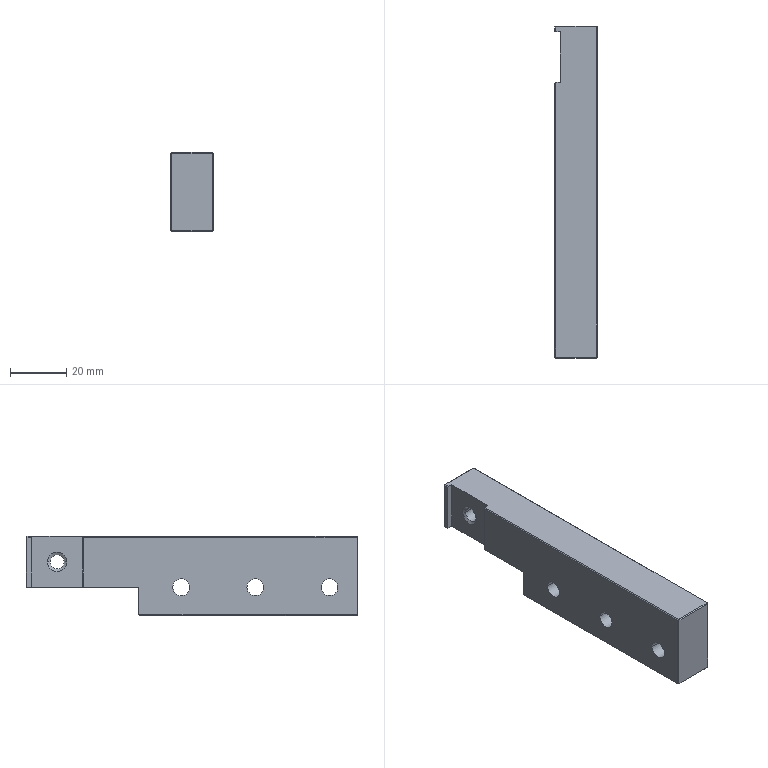Part | NX | 1 solid | 37 faces | box 15 x 117.567 x 28 mm | volume 41173 mm3 | plane 27 | cylinder 8 | cone 2 | commonest cylinder face diameters 6 x6 5 x2
STEP:
#1=CARTESIAN_POINT('',(-190.3,-54.817,-9.2));
#2=VERTEX_POINT('',#1);
#3=CARTESIAN_POINT('',(-204.7,-54.817,-9.2));
#4=VERTEX_POINT('',#3);
#5=CARTESIAN_POINT('',(-197.5,-54.817,-9.2));
#6=DIRECTION('',(-1.,0.,0.));
#7=VECTOR('',#6,1000.);
#8=LINE('',#5,#7);
#9=EDGE_CURVE('',#2,#4,#8,.T.);
#10=ORIENTED_EDGE('',*,*,#9,.F.);
#11=CARTESIAN_POINT('',(-190.3,-54.817,18.2));
#12=VERTEX_POINT('',#11);
#13=CARTESIAN_POINT('',(-190.3,-54.817,4.5));
#14=DIRECTION('',(0.,0.,-1.));
#15=VECTOR('',#14,1000.);
#16=LINE('',#13,#15);
#17=EDGE_CURVE('',#12,#2,#16,.T.);
#18=ORIENTED_EDGE('',*,*,#17,.F.);
#19=CARTESIAN_POINT('',(-204.7,-54.817,18.2));
#20=VERTEX_POINT('',#19);
#21=CARTESIAN_POINT('',(-197.5,-54.817,18.2));
#22=DIRECTION('',(-1.,0.,0.));
#23=VECTOR('',#22,1000.);
#24=LINE('',#21,#23);
#25=EDGE_CURVE('',#12,#20,#24,.T.);
#26=ORIENTED_EDGE('',*,*,#25,.T.);
#27=CARTESIAN_POINT('',(-204.7,-54.817,4.5));
#28=DIRECTION('',(0.,0.,-1.));
#29=VECTOR('',#28,1000.);
#30=LINE('',#27,#29);
#31=EDGE_CURVE('',#20,#4,#30,.T.);
#32=ORIENTED_EDGE('',*,*,#31,.T.);
#33=EDGE_LOOP('',(#10,#18,#26,#32));
#34=FACE_BOUND('',#33,.T.);
#35=CARTESIAN_POINT('',(-190.,-54.817,10.5));
#36=DIRECTION('',(0.,-1.,0.));
#37=DIRECTION('',(0.,0.,-1.));
#38=AXIS2_PLACEMENT_3D('',#35,#36,#37);
#39=PLANE('',#38);
#40=ADVANCED_FACE('',(#34),#39,.T.);
#41=CARTESIAN_POINT('',(-190.3,-54.517,18.5));
#42=VERTEX_POINT('',#41);
#43=CARTESIAN_POINT('',(-190.3,62.45,18.5));
#44=VERTEX_POINT('',#43);
#45=CARTESIAN_POINT('',(-190.3,3.967,18.5));
#46=DIRECTION('',(0.,1.,0.));
#47=VECTOR('',#46,1000.);
#48=LINE('',#45,#47);
#49=EDGE_CURVE('',#42,#44,#48,.T.);
#50=ORIENTED_EDGE('',*,*,#49,.T.);
#51=CARTESIAN_POINT('',(-204.7,62.45,18.5));
#52=VERTEX_POINT('',#51);
#53=CARTESIAN_POINT('',(-197.5,62.45,18.5));
#54=DIRECTION('',(1.,0.,0.));
#55=VECTOR('',#54,1000.);
#56=LINE('',#53,#55);
#57=EDGE_CURVE('',#52,#44,#56,.T.);
#58=ORIENTED_EDGE('',*,*,#57,.F.);
#59=CARTESIAN_POINT('',(-204.7,60.75,18.5));
#60=VERTEX_POINT('',#59);
#61=CARTESIAN_POINT('',(-204.7,61.75,18.5));
#62=DIRECTION('',(0.,1.,0.));
#63=VECTOR('',#62,1000.);
#64=LINE('',#61,#63);
#65=EDGE_CURVE('',#60,#52,#64,.T.);
#66=ORIENTED_EDGE('',*,*,#65,.F.);
#67=CARTESIAN_POINT('',(-203.,60.75,18.5));
#68=VERTEX_POINT('',#67);
#69=CARTESIAN_POINT('',(-190.,60.75,18.5));
#70=DIRECTION('',(-1.,0.,0.));
#71=VECTOR('',#70,1000.);
#72=LINE('',#69,#71);
#73=EDGE_CURVE('',#68,#60,#72,.T.);
#74=ORIENTED_EDGE('',*,*,#73,.F.);
#75=CARTESIAN_POINT('',(-203.,42.75,18.5));
#76=VERTEX_POINT('',#75);
#77=CARTESIAN_POINT('',(-203.,21.496,18.5));
#78=DIRECTION('',(0.,-1.,0.));
#79=VECTOR('',#78,1000.);
#80=LINE('',#77,#79);
#81=EDGE_CURVE('',#68,#76,#80,.T.);
#82=ORIENTED_EDGE('',*,*,#81,.T.);
#83=CARTESIAN_POINT('',(-204.7,42.75,18.5));
#84=VERTEX_POINT('',#83);
#85=CARTESIAN_POINT('',(-190.,42.75,18.5));
#86=DIRECTION('',(1.,0.,0.));
#87=VECTOR('',#86,1000.);
#88=LINE('',#85,#87);
#89=EDGE_CURVE('',#84,#76,#88,.T.);
#90=ORIENTED_EDGE('',*,*,#89,.F.);
#91=CARTESIAN_POINT('',(-204.7,-54.517,18.5));
#92=VERTEX_POINT('',#91);
#93=CARTESIAN_POINT('',(-204.7,-6.033,18.5));
#94=DIRECTION('',(0.,1.,0.));
#95=VECTOR('',#94,1000.);
#96=LINE('',#93,#95);
#97=EDGE_CURVE('',#92,#84,#96,.T.);
#98=ORIENTED_EDGE('',*,*,#97,.F.);
#99=CARTESIAN_POINT('',(-197.5,-54.517,18.5));
#100=DIRECTION('',(-1.,0.,0.));
#101=VECTOR('',#100,1000.);
#102=LINE('',#99,#101);
#103=EDGE_CURVE('',#42,#92,#102,.T.);
#104=ORIENTED_EDGE('',*,*,#103,.F.);
#105=EDGE_LOOP('',(#50,#58,#66,#74,#82,#90,#98,#104));
#106=FACE_BOUND('',#105,.T.);
#107=CARTESIAN_POINT('',(-190.,42.75,18.5));
#108=DIRECTION('',(0.,0.,1.));
#109=DIRECTION('',(1.,0.,0.));
#110=AXIS2_PLACEMENT_3D('',#107,#108,#109);
#111=PLANE('',#110);
#112=ADVANCED_FACE('',(#106),#111,.T.);
#113=CARTESIAN_POINT('',(-205.,22.75,-9.2));
#114=VERTEX_POINT('',#113);
#115=CARTESIAN_POINT('',(-190.,22.75,-9.2));
#116=VERTEX_POINT('',#115);
#117=CARTESIAN_POINT('',(-197.5,22.75,-9.2));
#118=DIRECTION('',(1.,0.,0.));
#119=VECTOR('',#118,1000.);
#120=LINE('',#117,#119);
#121=EDGE_CURVE('',#114,#116,#120,.T.);
#122=ORIENTED_EDGE('',*,*,#121,.F.);
#123=CARTESIAN_POINT('',(-205.,22.75,0.5));
#124=VERTEX_POINT('',#123);
#125=CARTESIAN_POINT('',(-205.,22.75,29.147));
#126=DIRECTION('',(0.,0.,-1.));
#127=VECTOR('',#126,1000.);
#128=LINE('',#125,#127);
#129=EDGE_CURVE('',#124,#114,#128,.T.);
#130=ORIENTED_EDGE('',*,*,#129,.F.);
#131=CARTESIAN_POINT('',(-190.,22.75,0.5));
#132=VERTEX_POINT('',#131);
#133=CARTESIAN_POINT('',(-190.,22.75,0.5));
#134=DIRECTION('',(1.,0.,0.));
#135=VECTOR('',#134,1000.);
#136=LINE('',#133,#135);
#137=EDGE_CURVE('',#124,#132,#136,.T.);
#138=ORIENTED_EDGE('',*,*,#137,.T.);
#139=CARTESIAN_POINT('',(-190.,22.75,29.147));
#140=DIRECTION('',(0.,0.,-1.));
#141=VECTOR('',#140,1000.);
#142=LINE('',#139,#141);
#143=EDGE_CURVE('',#132,#116,#142,.T.);
#144=ORIENTED_EDGE('',*,*,#143,.T.);
#145=EDGE_LOOP('',(#122,#130,#138,#144));
#146=FACE_BOUND('',#145,.T.);
#147=CARTESIAN_POINT('',(-190.,22.75,-9.5));
#148=DIRECTION('',(0.,1.,0.));
#149=DIRECTION('',(1.,0.,0.));
#150=AXIS2_PLACEMENT_3D('',#147,#148,#149);
#151=PLANE('',#150);
#152=ADVANCED_FACE('',(#146),#151,.T.);
#153=CARTESIAN_POINT('',(-190.3,-54.517,-9.5));
#154=VERTEX_POINT('',#153);
#155=CARTESIAN_POINT('',(-190.3,22.45,-9.5));
#156=VERTEX_POINT('',#155);
#157=CARTESIAN_POINT('',(-190.3,-16.033,-9.5));
#158=DIRECTION('',(0.,1.,0.));
#159=VECTOR('',#158,1000.);
#160=LINE('',#157,#159);
#161=EDGE_CURVE('',#154,#156,#160,.T.);
#162=ORIENTED_EDGE('',*,*,#161,.F.);
#163=CARTESIAN_POINT('',(-204.7,-54.517,-9.5));
#164=VERTEX_POINT('',#163);
#165=CARTESIAN_POINT('',(-197.5,-54.517,-9.5));
#166=DIRECTION('',(-1.,0.,0.));
#167=VECTOR('',#166,1000.);
#168=LINE('',#165,#167);
#169=EDGE_CURVE('',#154,#164,#168,.T.);
#170=ORIENTED_EDGE('',*,*,#169,.T.);
#171=CARTESIAN_POINT('',(-204.7,22.45,-9.5));
#172=VERTEX_POINT('',#171);
#173=CARTESIAN_POINT('',(-204.7,-16.033,-9.5));
#174=DIRECTION('',(0.,1.,0.));
#175=VECTOR('',#174,1000.);
#176=LINE('',#173,#175);
#177=EDGE_CURVE('',#164,#172,#176,.T.);
#178=ORIENTED_EDGE('',*,*,#177,.T.);
#179=CARTESIAN_POINT('',(-197.5,22.45,-9.5));
#180=DIRECTION('',(1.,0.,0.));
#181=VECTOR('',#180,1000.);
#182=LINE('',#179,#181);
#183=EDGE_CURVE('',#172,#156,#182,.T.);
#184=ORIENTED_EDGE('',*,*,#183,.T.);
#185=EDGE_LOOP('',(#162,#170,#178,#184));
#186=FACE_BOUND('',#185,.T.);
#187=CARTESIAN_POINT('',(-190.,-54.817,-9.5));
#188=DIRECTION('',(0.,0.,-1.));
#189=DIRECTION('',(0.,-1.,0.));
#190=AXIS2_PLACEMENT_3D('',#187,#188,#189);
#191=PLANE('',#190);
#192=ADVANCED_FACE('',(#186),#191,.T.);
#193=ORIENTED_EDGE('',*,*,#137,.F.);
#194=CARTESIAN_POINT('',(-205.,42.45,0.5));
#195=VERTEX_POINT('',#194);
#196=CARTESIAN_POINT('',(-205.,21.496,0.5));
#197=DIRECTION('',(0.,1.,0.));
#198=VECTOR('',#197,1000.);
#199=LINE('',#196,#198);
#200=EDGE_CURVE('',#124,#195,#199,.T.);
#201=ORIENTED_EDGE('',*,*,#200,.T.);
#202=CARTESIAN_POINT('',(-204.7,42.75,0.5));
#203=VERTEX_POINT('',#202);
#204=CARTESIAN_POINT('',(-190.,57.45,0.5));
#205=DIRECTION('',(0.7071,0.7071,0.));
#206=VECTOR('',#205,1000.);
#207=LINE('',#204,#206);
#208=EDGE_CURVE('',#195,#203,#207,.T.);
#209=ORIENTED_EDGE('',*,*,#208,.T.);
#210=CARTESIAN_POINT('',(-203.,42.75,0.5));
#211=VERTEX_POINT('',#210);
#212=CARTESIAN_POINT('',(-190.,42.75,0.5));
#213=DIRECTION('',(-1.,0.,0.));
#214=VECTOR('',#213,1000.);
#215=LINE('',#212,#214);
#216=EDGE_CURVE('',#211,#203,#215,.T.);
#217=ORIENTED_EDGE('',*,*,#216,.F.);
#218=CARTESIAN_POINT('',(-203.,60.75,0.5));
#219=VERTEX_POINT('',#218);
#220=CARTESIAN_POINT('',(-203.,21.496,0.5));
#221=DIRECTION('',(0.,1.,0.));
#222=VECTOR('',#221,1000.);
#223=LINE('',#220,#222);
#224=EDGE_CURVE('',#211,#219,#223,.T.);
#225=ORIENTED_EDGE('',*,*,#224,.T.);
#226=CARTESIAN_POINT('',(-205.,60.75,0.5));
#227=VERTEX_POINT('',#226);
#228=CARTESIAN_POINT('',(-190.,60.75,0.5));
#229=DIRECTION('',(1.,0.,0.));
#230=VECTOR('',#229,1000.);
#231=LINE('',#228,#230);
#232=EDGE_CURVE('',#227,#219,#231,.T.);
#233=ORIENTED_EDGE('',*,*,#232,.F.);
#234=CARTESIAN_POINT('',(-205.,62.45,0.5));
#235=VERTEX_POINT('',#234);
#236=CARTESIAN_POINT('',(-205.,21.496,0.5));
#237=DIRECTION('',(0.,1.,0.));
#238=VECTOR('',#237,1000.);
#239=LINE('',#236,#238);
#240=EDGE_CURVE('',#227,#235,#239,.T.);
#241=ORIENTED_EDGE('',*,*,#240,.T.);
#242=CARTESIAN_POINT('',(-190.,62.45,0.5));
#243=VERTEX_POINT('',#242);
#244=CARTESIAN_POINT('',(-197.5,62.45,0.5));
#245=DIRECTION('',(1.,0.,0.));
#246=VECTOR('',#245,1000.);
#247=LINE('',#244,#246);
#248=EDGE_CURVE('',#235,#243,#247,.T.);
#249=ORIENTED_EDGE('',*,*,#248,.T.);
#250=CARTESIAN_POINT('',(-190.,21.496,0.5));
#251=DIRECTION('',(0.,1.,0.));
#252=VECTOR('',#251,1000.);
#253=LINE('',#250,#252);
#254=EDGE_CURVE('',#132,#243,#253,.T.);
#255=ORIENTED_EDGE('',*,*,#254,.F.);
#256=EDGE_LOOP('',(#193,#201,#209,#217,#225,#233,#241,#249,#255));
#257=FACE_BOUND('',#256,.T.);
#258=CARTESIAN_POINT('',(-205.,42.75,0.5));
#259=DIRECTION('',(0.,0.,-1.));
#260=DIRECTION('',(0.,-1.,0.));
#261=AXIS2_PLACEMENT_3D('',#258,#259,#260);
#262=PLANE('',#261);
#263=ADVANCED_FACE('',(#257),#262,.T.);
#264=CARTESIAN_POINT('',(-190.3,62.75,18.2));
#265=VERTEX_POINT('',#264);
#266=CARTESIAN_POINT('',(-190.3,62.75,0.8));
#267=VERTEX_POINT('',#266);
#268=CARTESIAN_POINT('',(-190.3,62.75,9.5));
#269=DIRECTION('',(0.,0.,-1.));
#270=VECTOR('',#269,1000.);
#271=LINE('',#268,#270);
#272=EDGE_CURVE('',#265,#267,#271,.T.);
#273=ORIENTED_EDGE('',*,*,#272,.T.);
#274=CARTESIAN_POINT('',(-204.7,62.75,0.8));
#275=VERTEX_POINT('',#274);
#276=CARTESIAN_POINT('',(-197.5,62.75,0.8));
#277=DIRECTION('',(1.,0.,0.));
#278=VECTOR('',#277,1000.);
#279=LINE('',#276,#278);
#280=EDGE_CURVE('',#275,#267,#279,.T.);
#281=ORIENTED_EDGE('',*,*,#280,.F.);
#282=CARTESIAN_POINT('',(-204.7,62.75,18.2));
#283=VERTEX_POINT('',#282);
#284=CARTESIAN_POINT('',(-204.7,62.75,9.5));
#285=DIRECTION('',(0.,0.,-1.));
#286=VECTOR('',#285,1000.);
#287=LINE('',#284,#286);
#288=EDGE_CURVE('',#283,#275,#287,.T.);
#289=ORIENTED_EDGE('',*,*,#288,.F.);
#290=CARTESIAN_POINT('',(-197.5,62.75,18.2));
#291=DIRECTION('',(1.,0.,0.));
#292=VECTOR('',#291,1000.);
#293=LINE('',#290,#292);
#294=EDGE_CURVE('',#283,#265,#293,.T.);
#295=ORIENTED_EDGE('',*,*,#294,.T.);
#296=EDGE_LOOP('',(#273,#281,#289,#295));
#297=FACE_BOUND('',#296,.T.);
#298=CARTESIAN_POINT('',(-198.847,62.75,5.404));
#299=DIRECTION('',(0.,1.,0.));
#300=DIRECTION('',(1.,0.,0.));
#301=AXIS2_PLACEMENT_3D('',#298,#299,#300);
#302=PLANE('',#301);
#303=ADVANCED_FACE('',(#297),#302,.T.);
#304=ORIENTED_EDGE('',*,*,#232,.T.);
#305=CARTESIAN_POINT('',(-203.,60.75,18.5));
#306=DIRECTION('',(0.,0.,-1.));
#307=VECTOR('',#306,1000.);
#308=LINE('',#305,#307);
#309=EDGE_CURVE('',#68,#219,#308,.T.);
#310=ORIENTED_EDGE('',*,*,#309,.F.);
#311=ORIENTED_EDGE('',*,*,#73,.T.);
#312=CARTESIAN_POINT('',(-205.,60.75,18.2));
#313=VERTEX_POINT('',#312);
#314=CARTESIAN_POINT('',(-190.,60.75,33.2));
#315=DIRECTION('',(-0.7071,0.,-0.7071));
#316=VECTOR('',#315,1000.);
#317=LINE('',#314,#316);
#318=EDGE_CURVE('',#60,#313,#317,.T.);
#319=ORIENTED_EDGE('',*,*,#318,.T.);
#320=CARTESIAN_POINT('',(-205.,60.75,29.147));
#321=DIRECTION('',(0.,0.,-1.));
#322=VECTOR('',#321,1000.);
#323=LINE('',#320,#322);
#324=EDGE_CURVE('',#313,#227,#323,.T.);
#325=ORIENTED_EDGE('',*,*,#324,.T.);
#326=EDGE_LOOP('',(#304,#310,#311,#319,#325));
#327=FACE_BOUND('',#326,.T.);
#328=CARTESIAN_POINT('',(-205.,60.75,18.5));
#329=DIRECTION('',(0.,1.,0.));
#330=DIRECTION('',(1.,0.,0.));
#331=AXIS2_PLACEMENT_3D('',#328,#329,#330);
#332=PLANE('',#331);
#333=ADVANCED_FACE('',(#327),#332,.F.);
#334=ORIENTED_EDGE('',*,*,#309,.T.);
#335=ORIENTED_EDGE('',*,*,#224,.F.);
#336=CARTESIAN_POINT('',(-203.,42.75,0.5));
#337=DIRECTION('',(0.,0.,1.));
#338=VECTOR('',#337,1000.);
#339=LINE('',#336,#338);
#340=EDGE_CURVE('',#211,#76,#339,.T.);
#341=ORIENTED_EDGE('',*,*,#340,.T.);
#342=ORIENTED_EDGE('',*,*,#81,.F.);
#343=EDGE_LOOP('',(#334,#335,#341,#342));
#344=FACE_BOUND('',#343,.T.);
#345=CARTESIAN_POINT('',(-203.,55.2,9.5));
#346=VERTEX_POINT('',#345);
#347=CARTESIAN_POINT('',(-203.,48.3,9.5));
#348=VERTEX_POINT('',#347);
#349=CARTESIAN_POINT('',(-203.,51.75,9.5));
#350=DIRECTION('',(-1.,0.,0.));
#351=DIRECTION('',(0.,-1.,0.));
#352=AXIS2_PLACEMENT_3D('',#349,#350,#351);
#353=CIRCLE('',#352,3.45);
#354=EDGE_CURVE('',#346,#348,#353,.T.);
#355=ORIENTED_EDGE('',*,*,#354,.F.);
#356=CARTESIAN_POINT('',(-203.,51.75,9.5));
#357=DIRECTION('',(-1.,0.,0.));
#358=DIRECTION('',(0.,-1.,0.));
#359=AXIS2_PLACEMENT_3D('',#356,#357,#358);
#360=CIRCLE('',#359,3.45);
#361=EDGE_CURVE('',#348,#346,#360,.T.);
#362=ORIENTED_EDGE('',*,*,#361,.F.);
#363=EDGE_LOOP('',(#355,#362));
#364=FACE_BOUND('',#363,.T.);
#365=CARTESIAN_POINT('',(-203.,52.251,12.817));
#366=DIRECTION('',(-1.,0.,0.));
#367=DIRECTION('',(0.,0.,1.));
#368=AXIS2_PLACEMENT_3D('',#365,#366,#367);
#369=PLANE('',#368);
#370=ADVANCED_FACE('',(#344,#364),#369,.T.);
#371=ORIENTED_EDGE('',*,*,#89,.T.);
#372=ORIENTED_EDGE('',*,*,#340,.F.);
#373=ORIENTED_EDGE('',*,*,#216,.T.);
#374=CARTESIAN_POINT('',(-204.7,42.75,9.5));
#375=DIRECTION('',(0.,0.,1.));
#376=VECTOR('',#375,1000.);
#377=LINE('',#374,#376);
#378=EDGE_CURVE('',#203,#84,#377,.T.);
#379=ORIENTED_EDGE('',*,*,#378,.T.);
#380=EDGE_LOOP('',(#371,#372,#373,#379));
#381=FACE_BOUND('',#380,.T.);
#382=CARTESIAN_POINT('',(-205.,42.75,0.5));
#383=DIRECTION('',(0.,-1.,0.));
#384=DIRECTION('',(0.,0.,-1.));
#385=AXIS2_PLACEMENT_3D('',#382,#383,#384);
#386=PLANE('',#385);
#387=ADVANCED_FACE('',(#381),#386,.F.);
#388=CARTESIAN_POINT('',(-202.452,54.25,9.5));
#389=VERTEX_POINT('',#388);
#390=CARTESIAN_POINT('',(-202.452,49.25,9.5));
#391=VERTEX_POINT('',#390);
#392=CARTESIAN_POINT('',(-202.452,51.75,9.5));
#393=DIRECTION('',(-1.,0.,0.));
#394=DIRECTION('',(0.,-1.,0.));
#395=AXIS2_PLACEMENT_3D('',#392,#393,#394);
#396=CIRCLE('',#395,2.5);
#397=EDGE_CURVE('',#389,#391,#396,.T.);
#398=ORIENTED_EDGE('',*,*,#397,.T.);
#399=CARTESIAN_POINT('',(-190.,49.25,9.5));
#400=VERTEX_POINT('',#399);
#401=CARTESIAN_POINT('',(-203.,49.25,9.5));
#402=DIRECTION('',(-1.,0.,0.));
#403=VECTOR('',#402,1000.);
#404=LINE('',#401,#403);
#405=EDGE_CURVE('',#391,#400,#404,.F.);
#406=ORIENTED_EDGE('',*,*,#405,.T.);
#407=CARTESIAN_POINT('',(-190.,54.25,9.5));
#408=VERTEX_POINT('',#407);
#409=CARTESIAN_POINT('',(-190.,51.75,9.5));
#410=DIRECTION('',(-1.,0.,0.));
#411=DIRECTION('',(0.,-1.,0.));
#412=AXIS2_PLACEMENT_3D('',#409,#410,#411);
#413=CIRCLE('',#412,2.5);
#414=EDGE_CURVE('',#408,#400,#413,.T.);
#415=ORIENTED_EDGE('',*,*,#414,.F.);
#416=CARTESIAN_POINT('',(-203.,54.25,9.5));
#417=DIRECTION('',(-1.,0.,0.));
#418=VECTOR('',#417,1000.);
#419=LINE('',#416,#418);
#420=EDGE_CURVE('',#389,#408,#419,.F.);
#421=ORIENTED_EDGE('',*,*,#420,.F.);
#422=EDGE_LOOP('',(#398,#406,#415,#421));
#423=FACE_BOUND('',#422,.T.);
#424=CARTESIAN_POINT('',(-203.,51.75,9.5));
#425=DIRECTION('',(-1.,0.,0.));
#426=DIRECTION('',(0.,-1.,0.));
#427=AXIS2_PLACEMENT_3D('',#424,#425,#426);
#428=CYLINDRICAL_SURFACE('',#427,2.5);
#429=ADVANCED_FACE('',(#423),#428,.F.);
#430=ORIENTED_EDGE('',*,*,#397,.F.);
#431=CARTESIAN_POINT('',(-202.452,54.25,9.5));
#432=DIRECTION('',(-0.5,0.866,0.));
#433=VECTOR('',#432,1000.);
#434=LINE('',#431,#433);
#435=EDGE_CURVE('',#346,#389,#434,.F.);
#436=ORIENTED_EDGE('',*,*,#435,.F.);
#437=ORIENTED_EDGE('',*,*,#354,.T.);
#438=CARTESIAN_POINT('',(-202.452,49.25,9.5));
#439=DIRECTION('',(-0.5,-0.866,0.));
#440=VECTOR('',#439,1000.);
#441=LINE('',#438,#440);
#442=EDGE_CURVE('',#348,#391,#441,.F.);
#443=ORIENTED_EDGE('',*,*,#442,.T.);
#444=EDGE_LOOP('',(#430,#436,#437,#443));
#445=FACE_BOUND('',#444,.T.);
#446=CARTESIAN_POINT('',(-202.452,51.75,9.5));
#447=DIRECTION('',(-1.,0.,0.));
#448=DIRECTION('',(0.,-1.,0.));
#449=AXIS2_PLACEMENT_3D('',#446,#447,#448);
#450=CONICAL_SURFACE('',#449,2.5,1.047);
#451=ADVANCED_FACE('',(#445),#450,.F.);
#452=ORIENTED_EDGE('',*,*,#294,.F.);
#453=CARTESIAN_POINT('',(-204.85,62.6,18.35));
#454=VERTEX_POINT('',#453);
#455=CARTESIAN_POINT('',(-190.,77.45,3.5));
#456=DIRECTION('',(0.5774,0.5774,-0.5774));
#457=VECTOR('',#456,1000.);
#458=LINE('',#455,#457);
#459=EDGE_CURVE('',#454,#283,#458,.T.);
#460=ORIENTED_EDGE('',*,*,#459,.F.);
#461=CARTESIAN_POINT('',(-194.053,51.803,29.147));
#462=DIRECTION('',(-0.5774,0.5774,-0.5774));
#463=VECTOR('',#462,1000.);
#464=LINE('',#461,#463);
#465=EDGE_CURVE('',#52,#454,#464,.T.);
#466=ORIENTED_EDGE('',*,*,#465,.F.);
#467=ORIENTED_EDGE('',*,*,#57,.T.);
#468=CARTESIAN_POINT('',(-190.15,62.6,18.35));
#469=VERTEX_POINT('',#468);
#470=CARTESIAN_POINT('',(-200.947,51.803,29.147));
#471=DIRECTION('',(-0.5774,-0.5774,0.5774));
#472=VECTOR('',#471,1000.);
#473=LINE('',#470,#472);
#474=EDGE_CURVE('',#469,#44,#473,.T.);
#475=ORIENTED_EDGE('',*,*,#474,.F.);
#476=CARTESIAN_POINT('',(-190.,62.45,18.5));
#477=DIRECTION('',(-0.5774,0.5774,-0.5774));
#478=VECTOR('',#477,1000.);
#479=LINE('',#476,#478);
#480=EDGE_CURVE('',#469,#265,#479,.T.);
#481=ORIENTED_EDGE('',*,*,#480,.T.);
#482=EDGE_LOOP('',(#452,#460,#466,#467,#475,#481));
#483=FACE_BOUND('',#482,.T.);
#484=CARTESIAN_POINT('',(-197.5,62.6,18.35));
#485=DIRECTION('',(0.,0.7071,0.7071));
#486=DIRECTION('',(1.,0.,0.));
#487=AXIS2_PLACEMENT_3D('',#484,#485,#486);
#488=PLANE('',#487);
#489=ADVANCED_FACE('',(#483),#488,.T.);
#490=ORIENTED_EDGE('',*,*,#280,.T.);
#491=CARTESIAN_POINT('',(-190.,62.45,0.5));
#492=DIRECTION('',(-0.5774,0.5774,0.5774));
#493=VECTOR('',#492,1000.);
#494=LINE('',#491,#493);
#495=EDGE_CURVE('',#243,#267,#494,.T.);
#496=ORIENTED_EDGE('',*,*,#495,.F.);
#497=ORIENTED_EDGE('',*,*,#248,.F.);
#498=CARTESIAN_POINT('',(-190.,77.45,15.5));
#499=DIRECTION('',(0.5774,0.5774,0.5774));
#500=VECTOR('',#499,1000.);
#501=LINE('',#498,#500);
#502=EDGE_CURVE('',#235,#275,#501,.T.);
#503=ORIENTED_EDGE('',*,*,#502,.T.);
#504=EDGE_LOOP('',(#490,#496,#497,#503));
#505=FACE_BOUND('',#504,.T.);
#506=CARTESIAN_POINT('',(-197.5,62.6,0.65));
#507=DIRECTION('',(0.,-0.7071,0.7071));
#508=DIRECTION('',(-1.,0.,0.));
#509=AXIS2_PLACEMENT_3D('',#506,#507,#508);
#510=PLANE('',#509);
#511=ADVANCED_FACE('',(#505),#510,.F.);
#512=ORIENTED_EDGE('',*,*,#288,.T.);
#513=ORIENTED_EDGE('',*,*,#502,.F.);
#514=CARTESIAN_POINT('',(-205.,62.45,18.2));
#515=VERTEX_POINT('',#514);
#516=CARTESIAN_POINT('',(-205.,62.45,9.5));
#517=DIRECTION('',(0.,0.,-1.));
#518=VECTOR('',#517,1000.);
#519=LINE('',#516,#518);
#520=EDGE_CURVE('',#515,#235,#519,.T.);
#521=ORIENTED_EDGE('',*,*,#520,.F.);
#522=CARTESIAN_POINT('',(-190.,77.45,33.2));
#523=DIRECTION('',(0.5774,0.5774,0.5774));
#524=VECTOR('',#523,1000.);
#525=LINE('',#522,#524);
#526=EDGE_CURVE('',#515,#454,#525,.T.);
#527=ORIENTED_EDGE('',*,*,#526,.T.);
#528=ORIENTED_EDGE('',*,*,#459,.T.);
#529=EDGE_LOOP('',(#512,#513,#521,#527,#528));
#530=FACE_BOUND('',#529,.T.);
#531=CARTESIAN_POINT('',(-204.85,62.6,9.5));
#532=DIRECTION('',(0.7071,-0.7071,0.));
#533=DIRECTION('',(0.,0.,-1.));
#534=AXIS2_PLACEMENT_3D('',#531,#532,#533);
#535=PLANE('',#534);
#536=ADVANCED_FACE('',(#530),#535,.F.);
#537=ORIENTED_EDGE('',*,*,#272,.F.);
#538=ORIENTED_EDGE('',*,*,#480,.F.);
#539=CARTESIAN_POINT('',(-190.,62.45,18.2));
#540=VERTEX_POINT('',#539);
#541=CARTESIAN_POINT('',(-200.947,73.397,29.147));
#542=DIRECTION('',(0.5774,-0.5774,-0.5774));
#543=VECTOR('',#542,1000.);
#544=LINE('',#541,#543);
#545=EDGE_CURVE('',#469,#540,#544,.T.);
#546=ORIENTED_EDGE('',*,*,#545,.T.);
#547=CARTESIAN_POINT('',(-190.,62.45,9.5));
#548=DIRECTION('',(0.,0.,-1.));
#549=VECTOR('',#548,1000.);
#550=LINE('',#547,#549);
#551=EDGE_CURVE('',#540,#243,#550,.T.);
#552=ORIENTED_EDGE('',*,*,#551,.T.);
#553=ORIENTED_EDGE('',*,*,#495,.T.);
#554=EDGE_LOOP('',(#537,#538,#546,#552,#553));
#555=FACE_BOUND('',#554,.T.);
#556=CARTESIAN_POINT('',(-190.15,62.6,9.5));
#557=DIRECTION('',(0.7071,0.7071,0.));
#558=DIRECTION('',(0.,0.,-1.));
#559=AXIS2_PLACEMENT_3D('',#556,#557,#558);
#560=PLANE('',#559);
#561=ADVANCED_FACE('',(#555),#560,.T.);
#562=ORIENTED_EDGE('',*,*,#121,.T.);
#563=CARTESIAN_POINT('',(-191.254,21.496,-10.454));
#564=DIRECTION('',(0.5774,0.5774,0.5774));
#565=VECTOR('',#564,1000.);
#566=LINE('',#563,#565);
#567=EDGE_CURVE('',#156,#116,#566,.T.);
#568=ORIENTED_EDGE('',*,*,#567,.F.);
#569=ORIENTED_EDGE('',*,*,#183,.F.);
#570=CARTESIAN_POINT('',(-190.,7.75,-24.2));
#571=DIRECTION('',(-0.5774,0.5774,0.5774));
#572=VECTOR('',#571,1000.);
#573=LINE('',#570,#572);
#574=EDGE_CURVE('',#172,#114,#573,.T.);
#575=ORIENTED_EDGE('',*,*,#574,.T.);
#576=EDGE_LOOP('',(#562,#568,#569,#575));
#577=FACE_BOUND('',#576,.T.);
#578=CARTESIAN_POINT('',(-197.5,22.6,-9.35));
#579=DIRECTION('',(0.,-0.7071,0.7071));
#580=DIRECTION('',(-1.,0.,0.));
#581=AXIS2_PLACEMENT_3D('',#578,#579,#580);
#582=PLANE('',#581);
#583=ADVANCED_FACE('',(#577),#582,.F.);
#584=ORIENTED_EDGE('',*,*,#25,.F.);
#585=CARTESIAN_POINT('',(-190.15,-54.667,18.35));
#586=VERTEX_POINT('',#585);
#587=CARTESIAN_POINT('',(-179.353,-43.87,29.147));
#588=DIRECTION('',(0.5774,0.5774,0.5774));
#589=VECTOR('',#588,1000.);
#590=LINE('',#587,#589);
#591=EDGE_CURVE('',#12,#586,#590,.T.);
#592=ORIENTED_EDGE('',*,*,#591,.T.);
#593=CARTESIAN_POINT('',(-200.947,-43.87,29.147));
#594=DIRECTION('',(-0.5774,0.5774,0.5774));
#595=VECTOR('',#594,1000.);
#596=LINE('',#593,#595);
#597=EDGE_CURVE('',#586,#42,#596,.T.);
#598=ORIENTED_EDGE('',*,*,#597,.T.);
#599=ORIENTED_EDGE('',*,*,#103,.T.);
#600=CARTESIAN_POINT('',(-204.85,-54.667,18.35));
#601=VERTEX_POINT('',#600);
#602=CARTESIAN_POINT('',(-194.053,-43.87,29.147));
#603=DIRECTION('',(0.5774,0.5774,0.5774));
#604=VECTOR('',#603,1000.);
#605=LINE('',#602,#604);
#606=EDGE_CURVE('',#601,#92,#605,.T.);
#607=ORIENTED_EDGE('',*,*,#606,.F.);
#608=CARTESIAN_POINT('',(-190.,-69.517,3.5));
#609=DIRECTION('',(0.5774,-0.5774,-0.5774));
#610=VECTOR('',#609,1000.);
#611=LINE('',#608,#610);
#612=EDGE_CURVE('',#601,#20,#611,.T.);
#613=ORIENTED_EDGE('',*,*,#612,.T.);
#614=EDGE_LOOP('',(#584,#592,#598,#599,#607,#613));
#615=FACE_BOUND('',#614,.T.);
#616=CARTESIAN_POINT('',(-197.5,-54.667,18.35));
#617=DIRECTION('',(0.,-0.7071,0.7071));
#618=DIRECTION('',(-1.,0.,0.));
#619=AXIS2_PLACEMENT_3D('',#616,#617,#618);
#620=PLANE('',#619);
#621=ADVANCED_FACE('',(#615),#620,.T.);
#622=ORIENTED_EDGE('',*,*,#9,.T.);
#623=CARTESIAN_POINT('',(-204.85,-54.667,-9.35));
#624=VERTEX_POINT('',#623);
#625=CARTESIAN_POINT('',(-190.,-69.517,5.5));
#626=DIRECTION('',(0.5774,-0.5774,0.5774));
#627=VECTOR('',#626,1000.);
#628=LINE('',#625,#627);
#629=EDGE_CURVE('',#624,#4,#628,.T.);
#630=ORIENTED_EDGE('',*,*,#629,.F.);
#631=CARTESIAN_POINT('',(-190.,-39.817,-24.2));
#632=DIRECTION('',(-0.5774,-0.5774,0.5774));
#633=VECTOR('',#632,1000.);
#634=LINE('',#631,#633);
#635=EDGE_CURVE('',#164,#624,#634,.T.);
#636=ORIENTED_EDGE('',*,*,#635,.F.);
#637=ORIENTED_EDGE('',*,*,#169,.F.);
#638=CARTESIAN_POINT('',(-190.15,-54.667,-9.35));
#639=VERTEX_POINT('',#638);
#640=CARTESIAN_POINT('',(-190.,-54.817,-9.2));
#641=DIRECTION('',(0.5774,-0.5774,0.5774));
#642=VECTOR('',#641,1000.);
#643=LINE('',#640,#642);
#644=EDGE_CURVE('',#154,#639,#643,.T.);
#645=ORIENTED_EDGE('',*,*,#644,.T.);
#646=CARTESIAN_POINT('',(-190.,-54.517,-9.5));
#647=DIRECTION('',(-0.5774,-0.5774,0.5774));
#648=VECTOR('',#647,1000.);
#649=LINE('',#646,#648);
#650=EDGE_CURVE('',#639,#2,#649,.T.);
#651=ORIENTED_EDGE('',*,*,#650,.T.);
#652=EDGE_LOOP('',(#622,#630,#636,#637,#645,#651));
#653=FACE_BOUND('',#652,.T.);
#654=CARTESIAN_POINT('',(-197.5,-54.667,-9.35));
#655=DIRECTION('',(0.,0.7071,0.7071));
#656=DIRECTION('',(1.,0.,0.));
#657=AXIS2_PLACEMENT_3D('',#654,#655,#656);
#658=PLANE('',#657);
#659=ADVANCED_FACE('',(#653),#658,.F.);
#660=ORIENTED_EDGE('',*,*,#405,.F.);
#661=CARTESIAN_POINT('',(-202.452,51.75,9.5));
#662=DIRECTION('',(-1.,0.,0.));
#663=DIRECTION('',(0.,-1.,0.));
#664=AXIS2_PLACEMENT_3D('',#661,#662,#663);
#665=CIRCLE('',#664,2.5);
#666=EDGE_CURVE('',#391,#389,#665,.T.);
#667=ORIENTED_EDGE('',*,*,#666,.T.);
#668=ORIENTED_EDGE('',*,*,#420,.T.);
#669=CARTESIAN_POINT('',(-190.,51.75,9.5));
#670=DIRECTION('',(-1.,0.,0.));
#671=DIRECTION('',(0.,-1.,0.));
#672=AXIS2_PLACEMENT_3D('',#669,#670,#671);
#673=CIRCLE('',#672,2.5);
#674=EDGE_CURVE('',#400,#408,#673,.T.);
#675=ORIENTED_EDGE('',*,*,#674,.F.);
#676=EDGE_LOOP('',(#660,#667,#668,#675));
#677=FACE_BOUND('',#676,.T.);
#678=CARTESIAN_POINT('',(-203.,51.75,9.5));
#679=DIRECTION('',(-1.,0.,0.));
#680=DIRECTION('',(0.,-1.,0.));
#681=AXIS2_PLACEMENT_3D('',#678,#679,#680);
#682=CYLINDRICAL_SURFACE('',#681,2.5);
#683=ADVANCED_FACE('',(#677),#682,.F.);
#684=ORIENTED_EDGE('',*,*,#442,.F.);
#685=ORIENTED_EDGE('',*,*,#361,.T.);
#686=ORIENTED_EDGE('',*,*,#435,.T.);
#687=ORIENTED_EDGE('',*,*,#666,.F.);
#688=EDGE_LOOP('',(#684,#685,#686,#687));
#689=FACE_BOUND('',#688,.T.);
#690=CARTESIAN_POINT('',(-202.452,51.75,9.5));
#691=DIRECTION('',(-1.,0.,0.));
#692=DIRECTION('',(0.,-1.,0.));
#693=AXIS2_PLACEMENT_3D('',#690,#691,#692);
#694=CONICAL_SURFACE('',#693,2.5,1.047);
#695=ADVANCED_FACE('',(#689),#694,.F.);
#696=CARTESIAN_POINT('',(-205.,-21.5,0.5));
#697=VERTEX_POINT('',#696);
#698=CARTESIAN_POINT('',(-205.,-15.5,0.5));
#699=VERTEX_POINT('',#698);
#700=CARTESIAN_POINT('',(-205.,-18.5,0.5));
#701=DIRECTION('',(1.,0.,0.));
#702=DIRECTION('',(0.,1.,0.));
#703=AXIS2_PLACEMENT_3D('',#700,#701,#702);
#704=CIRCLE('',#703,3.);
#705=EDGE_CURVE('',#697,#699,#704,.T.);
#706=ORIENTED_EDGE('',*,*,#705,.F.);
#707=CARTESIAN_POINT('',(-190.,-21.5,0.5));
#708=VERTEX_POINT('',#707);
#709=CARTESIAN_POINT('',(-190.,-21.5,0.5));
#710=DIRECTION('',(1.,0.,0.));
#711=VECTOR('',#710,1000.);
#712=LINE('',#709,#711);
#713=EDGE_CURVE('',#697,#708,#712,.T.);
#714=ORIENTED_EDGE('',*,*,#713,.T.);
#715=CARTESIAN_POINT('',(-190.,-15.5,0.5));
#716=VERTEX_POINT('',#715);
#717=CARTESIAN_POINT('',(-190.,-18.5,0.5));
#718=DIRECTION('',(1.,0.,0.));
#719=DIRECTION('',(0.,1.,0.));
#720=AXIS2_PLACEMENT_3D('',#717,#718,#719);
#721=CIRCLE('',#720,3.);
#722=EDGE_CURVE('',#708,#716,#721,.T.);
#723=ORIENTED_EDGE('',*,*,#722,.T.);
#724=CARTESIAN_POINT('',(-190.,-15.5,0.5));
#725=DIRECTION('',(1.,0.,0.));
#726=VECTOR('',#725,1000.);
#727=LINE('',#724,#726);
#728=EDGE_CURVE('',#699,#716,#727,.T.);
#729=ORIENTED_EDGE('',*,*,#728,.F.);
#730=EDGE_LOOP('',(#706,#714,#723,#729));
#731=FACE_BOUND('',#730,.T.);
#732=CARTESIAN_POINT('',(-190.,-18.5,0.5));
#733=DIRECTION('',(1.,0.,0.));
#734=DIRECTION('',(0.,1.,0.));
#735=AXIS2_PLACEMENT_3D('',#732,#733,#734);
#736=CYLINDRICAL_SURFACE('',#735,3.);
#737=ADVANCED_FACE('',(#731),#736,.F.);
#738=ORIENTED_EDGE('',*,*,#728,.T.);
#739=CARTESIAN_POINT('',(-190.,-18.5,0.5));
#740=DIRECTION('',(1.,0.,0.));
#741=DIRECTION('',(0.,1.,0.));
#742=AXIS2_PLACEMENT_3D('',#739,#740,#741);
#743=CIRCLE('',#742,3.);
#744=EDGE_CURVE('',#716,#708,#743,.T.);
#745=ORIENTED_EDGE('',*,*,#744,.T.);
#746=ORIENTED_EDGE('',*,*,#713,.F.);
#747=CARTESIAN_POINT('',(-205.,-18.5,0.5));
#748=DIRECTION('',(1.,0.,0.));
#749=DIRECTION('',(0.,1.,0.));
#750=AXIS2_PLACEMENT_3D('',#747,#748,#749);
#751=CIRCLE('',#750,3.);
#752=EDGE_CURVE('',#699,#697,#751,.T.);
#753=ORIENTED_EDGE('',*,*,#752,.F.);
#754=EDGE_LOOP('',(#738,#745,#746,#753));
#755=FACE_BOUND('',#754,.T.);
#756=CARTESIAN_POINT('',(-190.,-18.5,0.5));
#757=DIRECTION('',(1.,0.,0.));
#758=DIRECTION('',(0.,1.,0.));
#759=AXIS2_PLACEMENT_3D('',#756,#757,#758);
#760=CYLINDRICAL_SURFACE('',#759,3.);
#761=ADVANCED_FACE('',(#755),#760,.F.);
#762=CARTESIAN_POINT('',(-205.,-47.75,0.5));
#763=VERTEX_POINT('',#762);
#764=CARTESIAN_POINT('',(-205.,-41.75,0.5));
#765=VERTEX_POINT('',#764);
#766=CARTESIAN_POINT('',(-205.,-44.75,0.5));
#767=DIRECTION('',(1.,0.,0.));
#768=DIRECTION('',(0.,1.,0.));
#769=AXIS2_PLACEMENT_3D('',#766,#767,#768);
#770=CIRCLE('',#769,3.);
#771=EDGE_CURVE('',#763,#765,#770,.T.);
#772=ORIENTED_EDGE('',*,*,#771,.F.);
#773=CARTESIAN_POINT('',(-190.,-47.75,0.5));
#774=VERTEX_POINT('',#773);
#775=CARTESIAN_POINT('',(-190.,-47.75,0.5));
#776=DIRECTION('',(1.,0.,0.));
#777=VECTOR('',#776,1000.);
#778=LINE('',#775,#777);
#779=EDGE_CURVE('',#763,#774,#778,.T.);
#780=ORIENTED_EDGE('',*,*,#779,.T.);
#781=CARTESIAN_POINT('',(-190.,-41.75,0.5));
#782=VERTEX_POINT('',#781);
#783=CARTESIAN_POINT('',(-190.,-44.75,0.5));
#784=DIRECTION('',(1.,0.,0.));
#785=DIRECTION('',(0.,1.,0.));
#786=AXIS2_PLACEMENT_3D('',#783,#784,#785);
#787=CIRCLE('',#786,3.);
#788=EDGE_CURVE('',#774,#782,#787,.T.);
#789=ORIENTED_EDGE('',*,*,#788,.T.);
#790=CARTESIAN_POINT('',(-190.,-41.75,0.5));
#791=DIRECTION('',(1.,0.,0.));
#792=VECTOR('',#791,1000.);
#793=LINE('',#790,#792);
#794=EDGE_CURVE('',#765,#782,#793,.T.);
#795=ORIENTED_EDGE('',*,*,#794,.F.);
#796=EDGE_LOOP('',(#772,#780,#789,#795));
#797=FACE_BOUND('',#796,.T.);
#798=CARTESIAN_POINT('',(-190.,-44.75,0.5));
#799=DIRECTION('',(1.,0.,0.));
#800=DIRECTION('',(0.,1.,0.));
#801=AXIS2_PLACEMENT_3D('',#798,#799,#800);
#802=CYLINDRICAL_SURFACE('',#801,3.);
#803=ADVANCED_FACE('',(#797),#802,.F.);
#804=ORIENTED_EDGE('',*,*,#794,.T.);
#805=CARTESIAN_POINT('',(-190.,-44.75,0.5));
#806=DIRECTION('',(1.,0.,0.));
#807=DIRECTION('',(0.,1.,0.));
#808=AXIS2_PLACEMENT_3D('',#805,#806,#807);
#809=CIRCLE('',#808,3.);
#810=EDGE_CURVE('',#782,#774,#809,.T.);
#811=ORIENTED_EDGE('',*,*,#810,.T.);
#812=ORIENTED_EDGE('',*,*,#779,.F.);
#813=CARTESIAN_POINT('',(-205.,-44.75,0.5));
#814=DIRECTION('',(1.,0.,0.));
#815=DIRECTION('',(0.,1.,0.));
#816=AXIS2_PLACEMENT_3D('',#813,#814,#815);
#817=CIRCLE('',#816,3.);
#818=EDGE_CURVE('',#765,#763,#817,.T.);
#819=ORIENTED_EDGE('',*,*,#818,.F.);
#820=EDGE_LOOP('',(#804,#811,#812,#819));
#821=FACE_BOUND('',#820,.T.);
#822=CARTESIAN_POINT('',(-190.,-44.75,0.5));
#823=DIRECTION('',(1.,0.,0.));
#824=DIRECTION('',(0.,1.,0.));
#825=AXIS2_PLACEMENT_3D('',#822,#823,#824);
#826=CYLINDRICAL_SURFACE('',#825,3.);
#827=ADVANCED_FACE('',(#821),#826,.F.);
#828=CARTESIAN_POINT('',(-205.,4.75,0.5));
#829=VERTEX_POINT('',#828);
#830=CARTESIAN_POINT('',(-205.,10.75,0.5));
#831=VERTEX_POINT('',#830);
#832=CARTESIAN_POINT('',(-205.,7.75,0.5));
#833=DIRECTION('',(1.,0.,0.));
#834=DIRECTION('',(0.,1.,0.));
#835=AXIS2_PLACEMENT_3D('',#832,#833,#834);
#836=CIRCLE('',#835,3.);
#837=EDGE_CURVE('',#829,#831,#836,.T.);
#838=ORIENTED_EDGE('',*,*,#837,.F.);
#839=CARTESIAN_POINT('',(-190.,4.75,0.5));
#840=VERTEX_POINT('',#839);
#841=CARTESIAN_POINT('',(-190.,4.75,0.5));
#842=DIRECTION('',(1.,0.,0.));
#843=VECTOR('',#842,1000.);
#844=LINE('',#841,#843);
#845=EDGE_CURVE('',#829,#840,#844,.T.);
#846=ORIENTED_EDGE('',*,*,#845,.T.);
#847=CARTESIAN_POINT('',(-190.,10.75,0.5));
#848=VERTEX_POINT('',#847);
#849=CARTESIAN_POINT('',(-190.,7.75,0.5));
#850=DIRECTION('',(1.,0.,0.));
#851=DIRECTION('',(0.,1.,0.));
#852=AXIS2_PLACEMENT_3D('',#849,#850,#851);
#853=CIRCLE('',#852,3.);
#854=EDGE_CURVE('',#840,#848,#853,.T.);
#855=ORIENTED_EDGE('',*,*,#854,.T.);
#856=CARTESIAN_POINT('',(-190.,10.75,0.5));
#857=DIRECTION('',(1.,0.,0.));
#858=VECTOR('',#857,1000.);
#859=LINE('',#856,#858);
#860=EDGE_CURVE('',#831,#848,#859,.T.);
#861=ORIENTED_EDGE('',*,*,#860,.F.);
#862=EDGE_LOOP('',(#838,#846,#855,#861));
#863=FACE_BOUND('',#862,.T.);
#864=CARTESIAN_POINT('',(-190.,7.75,0.5));
#865=DIRECTION('',(1.,0.,0.));
#866=DIRECTION('',(0.,1.,0.));
#867=AXIS2_PLACEMENT_3D('',#864,#865,#866);
#868=CYLINDRICAL_SURFACE('',#867,3.);
#869=ADVANCED_FACE('',(#863),#868,.F.);
#870=ORIENTED_EDGE('',*,*,#860,.T.);
#871=CARTESIAN_POINT('',(-190.,7.75,0.5));
#872=DIRECTION('',(1.,0.,0.));
#873=DIRECTION('',(0.,1.,0.));
#874=AXIS2_PLACEMENT_3D('',#871,#872,#873);
#875=CIRCLE('',#874,3.);
#876=EDGE_CURVE('',#848,#840,#875,.T.);
#877=ORIENTED_EDGE('',*,*,#876,.T.);
#878=ORIENTED_EDGE('',*,*,#845,.F.);
#879=CARTESIAN_POINT('',(-205.,7.75,0.5));
#880=DIRECTION('',(1.,0.,0.));
#881=DIRECTION('',(0.,1.,0.));
#882=AXIS2_PLACEMENT_3D('',#879,#880,#881);
#883=CIRCLE('',#882,3.);
#884=EDGE_CURVE('',#831,#829,#883,.T.);
#885=ORIENTED_EDGE('',*,*,#884,.F.);
#886=EDGE_LOOP('',(#870,#877,#878,#885));
#887=FACE_BOUND('',#886,.T.);
#888=CARTESIAN_POINT('',(-190.,7.75,0.5));
#889=DIRECTION('',(1.,0.,0.));
#890=DIRECTION('',(0.,1.,0.));
#891=AXIS2_PLACEMENT_3D('',#888,#889,#890);
#892=CYLINDRICAL_SURFACE('',#891,3.);
#893=ADVANCED_FACE('',(#887),#892,.F.);
#894=CARTESIAN_POINT('',(-205.,-54.517,18.2));
#895=VERTEX_POINT('',#894);
#896=CARTESIAN_POINT('',(-205.,-54.517,-9.2));
#897=VERTEX_POINT('',#896);
#898=CARTESIAN_POINT('',(-205.,-54.517,4.5));
#899=DIRECTION('',(0.,0.,-1.));
#900=VECTOR('',#899,1000.);
#901=LINE('',#898,#900);
#902=EDGE_CURVE('',#895,#897,#901,.T.);
#903=ORIENTED_EDGE('',*,*,#902,.F.);
#904=CARTESIAN_POINT('',(-205.,42.45,18.2));
#905=VERTEX_POINT('',#904);
#906=CARTESIAN_POINT('',(-205.,-6.033,18.2));
#907=DIRECTION('',(0.,1.,0.));
#908=VECTOR('',#907,1000.);
#909=LINE('',#906,#908);
#910=EDGE_CURVE('',#895,#905,#909,.T.);
#911=ORIENTED_EDGE('',*,*,#910,.T.);
#912=CARTESIAN_POINT('',(-205.,42.45,9.5));
#913=DIRECTION('',(0.,0.,1.));
#914=VECTOR('',#913,1000.);
#915=LINE('',#912,#914);
#916=EDGE_CURVE('',#195,#905,#915,.T.);
#917=ORIENTED_EDGE('',*,*,#916,.F.);
#918=ORIENTED_EDGE('',*,*,#200,.F.);
#919=ORIENTED_EDGE('',*,*,#129,.T.);
#920=CARTESIAN_POINT('',(-205.,-16.033,-9.2));
#921=DIRECTION('',(0.,1.,0.));
#922=VECTOR('',#921,1000.);
#923=LINE('',#920,#922);
#924=EDGE_CURVE('',#897,#114,#923,.T.);
#925=ORIENTED_EDGE('',*,*,#924,.F.);
#926=EDGE_LOOP('',(#903,#911,#917,#918,#919,#925));
#927=FACE_BOUND('',#926,.T.);
#928=ORIENTED_EDGE('',*,*,#837,.T.);
#929=ORIENTED_EDGE('',*,*,#884,.T.);
#930=EDGE_LOOP('',(#928,#929));
#931=FACE_BOUND('',#930,.T.);
#932=ORIENTED_EDGE('',*,*,#771,.T.);
#933=ORIENTED_EDGE('',*,*,#818,.T.);
#934=EDGE_LOOP('',(#932,#933));
#935=FACE_BOUND('',#934,.T.);
#936=ORIENTED_EDGE('',*,*,#705,.T.);
#937=ORIENTED_EDGE('',*,*,#752,.T.);
#938=EDGE_LOOP('',(#936,#937));
#939=FACE_BOUND('',#938,.T.);
#940=CARTESIAN_POINT('',(-205.,21.496,29.147));
#941=DIRECTION('',(-1.,0.,0.));
#942=DIRECTION('',(0.,0.,1.));
#943=AXIS2_PLACEMENT_3D('',#940,#941,#942);
#944=PLANE('',#943);
#945=ADVANCED_FACE('',(#927,#931,#935,#939),#944,.T.);
#946=CARTESIAN_POINT('',(-205.,61.75,18.2));
#947=DIRECTION('',(0.,1.,0.));
#948=VECTOR('',#947,1000.);
#949=LINE('',#946,#948);
#950=EDGE_CURVE('',#313,#515,#949,.T.);
#951=ORIENTED_EDGE('',*,*,#950,.T.);
#952=ORIENTED_EDGE('',*,*,#520,.T.);
#953=ORIENTED_EDGE('',*,*,#240,.F.);
#954=ORIENTED_EDGE('',*,*,#324,.F.);
#955=EDGE_LOOP('',(#951,#952,#953,#954));
#956=FACE_BOUND('',#955,.T.);
#957=CARTESIAN_POINT('',(-205.,21.496,29.147));
#958=DIRECTION('',(-1.,0.,0.));
#959=DIRECTION('',(0.,0.,1.));
#960=AXIS2_PLACEMENT_3D('',#957,#958,#959);
#961=PLANE('',#960);
#962=ADVANCED_FACE('',(#956),#961,.T.);
#963=ORIENTED_EDGE('',*,*,#910,.F.);
#964=CARTESIAN_POINT('',(-190.,-69.517,33.2));
#965=DIRECTION('',(-0.5774,0.5774,-0.5774));
#966=VECTOR('',#965,1000.);
#967=LINE('',#964,#966);
#968=EDGE_CURVE('',#601,#895,#967,.T.);
#969=ORIENTED_EDGE('',*,*,#968,.F.);
#970=ORIENTED_EDGE('',*,*,#606,.T.);
#971=ORIENTED_EDGE('',*,*,#97,.T.);
#972=CARTESIAN_POINT('',(-190.,57.45,33.2));
#973=DIRECTION('',(0.5774,0.5774,0.5774));
#974=VECTOR('',#973,1000.);
#975=LINE('',#972,#974);
#976=EDGE_CURVE('',#905,#84,#975,.T.);
#977=ORIENTED_EDGE('',*,*,#976,.F.);
#978=EDGE_LOOP('',(#963,#969,#970,#971,#977));
#979=FACE_BOUND('',#978,.T.);
#980=CARTESIAN_POINT('',(-204.85,-6.033,18.35));
#981=DIRECTION('',(-0.7071,0.,0.7071));
#982=DIRECTION('',(0.,1.,0.));
#983=AXIS2_PLACEMENT_3D('',#980,#981,#982);
#984=PLANE('',#983);
#985=ADVANCED_FACE('',(#979),#984,.T.);
#986=ORIENTED_EDGE('',*,*,#950,.F.);
#987=ORIENTED_EDGE('',*,*,#318,.F.);
#988=ORIENTED_EDGE('',*,*,#65,.T.);
#989=ORIENTED_EDGE('',*,*,#465,.T.);
#990=ORIENTED_EDGE('',*,*,#526,.F.);
#991=EDGE_LOOP('',(#986,#987,#988,#989,#990));
#992=FACE_BOUND('',#991,.T.);
#993=CARTESIAN_POINT('',(-204.85,61.75,18.35));
#994=DIRECTION('',(-0.7071,0.,0.7071));
#995=DIRECTION('',(0.,1.,0.));
#996=AXIS2_PLACEMENT_3D('',#993,#994,#995);
#997=PLANE('',#996);
#998=ADVANCED_FACE('',(#992),#997,.T.);
#999=ORIENTED_EDGE('',*,*,#924,.T.);
#1000=ORIENTED_EDGE('',*,*,#574,.F.);
#1001=ORIENTED_EDGE('',*,*,#177,.F.);
#1002=ORIENTED_EDGE('',*,*,#635,.T.);
#1003=CARTESIAN_POINT('',(-190.,-69.517,-24.2));
#1004=DIRECTION('',(-0.5774,0.5774,0.5774));
#1005=VECTOR('',#1004,1000.);
#1006=LINE('',#1003,#1005);
#1007=EDGE_CURVE('',#624,#897,#1006,.T.);
#1008=ORIENTED_EDGE('',*,*,#1007,.T.);
#1009=EDGE_LOOP('',(#999,#1000,#1001,#1002,#1008));
#1010=FACE_BOUND('',#1009,.T.);
#1011=CARTESIAN_POINT('',(-204.85,-16.033,-9.35));
#1012=DIRECTION('',(0.7071,0.,0.7071));
#1013=DIRECTION('',(0.,-1.,0.));
#1014=AXIS2_PLACEMENT_3D('',#1011,#1012,#1013);
#1015=PLANE('',#1014);
#1016=ADVANCED_FACE('',(#1010),#1015,.F.);
#1017=ORIENTED_EDGE('',*,*,#916,.T.);
#1018=ORIENTED_EDGE('',*,*,#976,.T.);
#1019=ORIENTED_EDGE('',*,*,#378,.F.);
#1020=ORIENTED_EDGE('',*,*,#208,.F.);
#1021=EDGE_LOOP('',(#1017,#1018,#1019,#1020));
#1022=FACE_BOUND('',#1021,.T.);
#1023=CARTESIAN_POINT('',(-204.85,42.6,9.5));
#1024=DIRECTION('',(0.7071,-0.7071,0.));
#1025=DIRECTION('',(0.,0.,-1.));
#1026=AXIS2_PLACEMENT_3D('',#1023,#1024,#1025);
#1027=PLANE('',#1026);
#1028=ADVANCED_FACE('',(#1022),#1027,.F.);
#1029=ORIENTED_EDGE('',*,*,#902,.T.);
#1030=ORIENTED_EDGE('',*,*,#1007,.F.);
#1031=ORIENTED_EDGE('',*,*,#629,.T.);
#1032=ORIENTED_EDGE('',*,*,#31,.F.);
#1033=ORIENTED_EDGE('',*,*,#612,.F.);
#1034=ORIENTED_EDGE('',*,*,#968,.T.);
#1035=EDGE_LOOP('',(#1029,#1030,#1031,#1032,#1033,#1034));
#1036=FACE_BOUND('',#1035,.T.);
#1037=CARTESIAN_POINT('',(-204.85,-54.667,4.5));
#1038=DIRECTION('',(0.7071,0.7071,0.));
#1039=DIRECTION('',(0.,0.,-1.));
#1040=AXIS2_PLACEMENT_3D('',#1037,#1038,#1039);
#1041=PLANE('',#1040);
#1042=ADVANCED_FACE('',(#1036),#1041,.F.);
#1043=CARTESIAN_POINT('',(-190.,-54.517,18.2));
#1044=VERTEX_POINT('',#1043);
#1045=CARTESIAN_POINT('',(-190.,-54.517,-9.2));
#1046=VERTEX_POINT('',#1045);
#1047=CARTESIAN_POINT('',(-190.,-54.517,4.5));
#1048=DIRECTION('',(0.,0.,-1.));
#1049=VECTOR('',#1048,1000.);
#1050=LINE('',#1047,#1049);
#1051=EDGE_CURVE('',#1044,#1046,#1050,.T.);
#1052=ORIENTED_EDGE('',*,*,#1051,.T.);
#1053=CARTESIAN_POINT('',(-190.,-16.033,-9.2));
#1054=DIRECTION('',(0.,1.,0.));
#1055=VECTOR('',#1054,1000.);
#1056=LINE('',#1053,#1055);
#1057=EDGE_CURVE('',#1046,#116,#1056,.T.);
#1058=ORIENTED_EDGE('',*,*,#1057,.T.);
#1059=ORIENTED_EDGE('',*,*,#143,.F.);
#1060=ORIENTED_EDGE('',*,*,#254,.T.);
#1061=ORIENTED_EDGE('',*,*,#551,.F.);
#1062=CARTESIAN_POINT('',(-190.,3.967,18.2));
#1063=DIRECTION('',(0.,1.,0.));
#1064=VECTOR('',#1063,1000.);
#1065=LINE('',#1062,#1064);
#1066=EDGE_CURVE('',#1044,#540,#1065,.T.);
#1067=ORIENTED_EDGE('',*,*,#1066,.F.);
#1068=EDGE_LOOP('',(#1052,#1058,#1059,#1060,#1061,#1067));
#1069=FACE_BOUND('',#1068,.T.);
#1070=ORIENTED_EDGE('',*,*,#854,.F.);
#1071=ORIENTED_EDGE('',*,*,#876,.F.);
#1072=EDGE_LOOP('',(#1070,#1071));
#1073=FACE_BOUND('',#1072,.T.);
#1074=ORIENTED_EDGE('',*,*,#414,.T.);
#1075=ORIENTED_EDGE('',*,*,#674,.T.);
#1076=EDGE_LOOP('',(#1074,#1075));
#1077=FACE_BOUND('',#1076,.T.);
#1078=ORIENTED_EDGE('',*,*,#788,.F.);
#1079=ORIENTED_EDGE('',*,*,#810,.F.);
#1080=EDGE_LOOP('',(#1078,#1079));
#1081=FACE_BOUND('',#1080,.T.);
#1082=ORIENTED_EDGE('',*,*,#722,.F.);
#1083=ORIENTED_EDGE('',*,*,#744,.F.);
#1084=EDGE_LOOP('',(#1082,#1083));
#1085=FACE_BOUND('',#1084,.T.);
#1086=CARTESIAN_POINT('',(-190.,21.496,29.147));
#1087=DIRECTION('',(-1.,0.,0.));
#1088=DIRECTION('',(0.,0.,1.));
#1089=AXIS2_PLACEMENT_3D('',#1086,#1087,#1088);
#1090=PLANE('',#1089);
#1091=ADVANCED_FACE('',(#1069,#1073,#1077,#1081,#1085),#1090,.F.);
#1092=ORIENTED_EDGE('',*,*,#1066,.T.);
#1093=ORIENTED_EDGE('',*,*,#545,.F.);
#1094=ORIENTED_EDGE('',*,*,#474,.T.);
#1095=ORIENTED_EDGE('',*,*,#49,.F.);
#1096=ORIENTED_EDGE('',*,*,#597,.F.);
#1097=CARTESIAN_POINT('',(-200.947,-65.464,29.147));
#1098=DIRECTION('',(-0.5774,-0.5774,0.5774));
#1099=VECTOR('',#1098,1000.);
#1100=LINE('',#1097,#1099);
#1101=EDGE_CURVE('',#1044,#586,#1100,.T.);
#1102=ORIENTED_EDGE('',*,*,#1101,.F.);
#1103=EDGE_LOOP('',(#1092,#1093,#1094,#1095,#1096,#1102));
#1104=FACE_BOUND('',#1103,.T.);
#1105=CARTESIAN_POINT('',(-190.15,3.967,18.35));
#1106=DIRECTION('',(-0.7071,0.,-0.7071));
#1107=DIRECTION('',(-0.7071,0.,0.7071));
#1108=AXIS2_PLACEMENT_3D('',#1105,#1106,#1107);
#1109=PLANE('',#1108);
#1110=ADVANCED_FACE('',(#1104),#1109,.F.);
#1111=ORIENTED_EDGE('',*,*,#1057,.F.);
#1112=CARTESIAN_POINT('',(-190.,-54.517,-9.2));
#1113=DIRECTION('',(-0.5774,-0.5774,-0.5774));
#1114=VECTOR('',#1113,1000.);
#1115=LINE('',#1112,#1114);
#1116=EDGE_CURVE('',#1046,#639,#1115,.T.);
#1117=ORIENTED_EDGE('',*,*,#1116,.T.);
#1118=ORIENTED_EDGE('',*,*,#644,.F.);
#1119=ORIENTED_EDGE('',*,*,#161,.T.);
#1120=ORIENTED_EDGE('',*,*,#567,.T.);
#1121=EDGE_LOOP('',(#1111,#1117,#1118,#1119,#1120));
#1122=FACE_BOUND('',#1121,.T.);
#1123=CARTESIAN_POINT('',(-190.15,-16.033,-9.35));
#1124=DIRECTION('',(0.7071,0.,-0.7071));
#1125=DIRECTION('',(0.,-1.,0.));
#1126=AXIS2_PLACEMENT_3D('',#1123,#1124,#1125);
#1127=PLANE('',#1126);
#1128=ADVANCED_FACE('',(#1122),#1127,.T.);
#1129=ORIENTED_EDGE('',*,*,#1051,.F.);
#1130=ORIENTED_EDGE('',*,*,#1101,.T.);
#1131=ORIENTED_EDGE('',*,*,#591,.F.);
#1132=ORIENTED_EDGE('',*,*,#17,.T.);
#1133=ORIENTED_EDGE('',*,*,#650,.F.);
#1134=ORIENTED_EDGE('',*,*,#1116,.F.);
#1135=EDGE_LOOP('',(#1129,#1130,#1131,#1132,#1133,#1134));
#1136=FACE_BOUND('',#1135,.T.);
#1137=CARTESIAN_POINT('',(-190.15,-54.667,4.5));
#1138=DIRECTION('',(0.7071,-0.7071,0.));
#1139=DIRECTION('',(0.,0.,-1.));
#1140=AXIS2_PLACEMENT_3D('',#1137,#1138,#1139);
#1141=PLANE('',#1140);
#1142=ADVANCED_FACE('',(#1136),#1141,.T.);
#1143=CLOSED_SHELL('',(#40,#112,#152,#192,#263,#303,#333,#370,#387,#429,#451,#489,#511,#536,#561,#583,#621,#659,#683,#695,#737,#761,#803,#827,#869,#893,#945,#962,#985,#998,#1016,#1028,#1042,#1091,#1110,#1128,#1142));
#1144=MANIFOLD_SOLID_BREP('',#1143);
#1145=(LENGTH_UNIT()NAMED_UNIT(*)SI_UNIT(.MILLI.,.METRE.));
#1146=UNCERTAINTY_MEASURE_WITH_UNIT(LENGTH_MEASURE(0.00001),#1145,'','');
#1147=(NAMED_UNIT(*)PLANE_ANGLE_UNIT()SI_UNIT($,.RADIAN.));
#1148=(NAMED_UNIT(*)SI_UNIT($,.STERADIAN.)SOLID_ANGLE_UNIT());
#1149=(GEOMETRIC_REPRESENTATION_CONTEXT(3)GLOBAL_UNCERTAINTY_ASSIGNED_CONTEXT((#1146))GLOBAL_UNIT_ASSIGNED_CONTEXT((#1145,#1147,#1148))REPRESENTATION_CONTEXT('',''));
#1150=ADVANCED_BREP_SHAPE_REPRESENTATION('',(#1144),#1149);